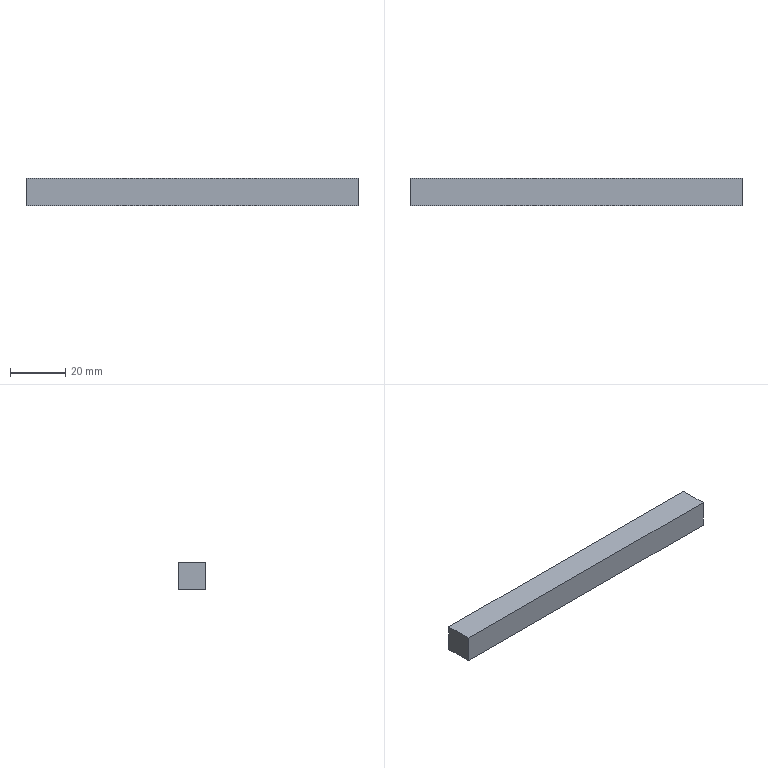Part | STEP file | X-Axis Clamp Block 1 | 1 solid | 6 faces | box 120 x 10 x 10 mm | volume 12000 mm3 | plane 6
STEP:
#1=CARTESIAN_POINT('',(160.919,-17.57,10.));
#2=VERTEX_POINT('',#1);
#3=CARTESIAN_POINT('',(160.919,-17.57,0.));
#4=VERTEX_POINT('',#3);
#5=CARTESIAN_POINT('',(160.919,-17.57,10.));
#6=DIRECTION('',(0.,0.,-1.));
#7=VECTOR('',#6,1000.);
#8=LINE('',#5,#7);
#9=EDGE_CURVE('',#2,#4,#8,.T.);
#10=ORIENTED_EDGE('',*,*,#9,.F.);
#11=CARTESIAN_POINT('',(40.919,-17.57,10.));
#12=VERTEX_POINT('',#11);
#13=CARTESIAN_POINT('',(40.919,-17.57,10.));
#14=DIRECTION('',(1.,0.,0.));
#15=VECTOR('',#14,1000.);
#16=LINE('',#13,#15);
#17=EDGE_CURVE('',#12,#2,#16,.T.);
#18=ORIENTED_EDGE('',*,*,#17,.F.);
#19=CARTESIAN_POINT('',(40.919,-17.57,0.));
#20=VERTEX_POINT('',#19);
#21=CARTESIAN_POINT('',(40.919,-17.57,10.));
#22=DIRECTION('',(0.,0.,1.));
#23=VECTOR('',#22,1000.);
#24=LINE('',#21,#23);
#25=EDGE_CURVE('',#20,#12,#24,.T.);
#26=ORIENTED_EDGE('',*,*,#25,.F.);
#27=CARTESIAN_POINT('',(40.919,-17.57,0.));
#28=DIRECTION('',(-1.,0.,0.));
#29=VECTOR('',#28,1000.);
#30=LINE('',#27,#29);
#31=EDGE_CURVE('',#4,#20,#30,.T.);
#32=ORIENTED_EDGE('',*,*,#31,.F.);
#33=EDGE_LOOP('',(#10,#18,#26,#32));
#34=FACE_OUTER_BOUND('',#33,.T.);
#35=CARTESIAN_POINT('',(40.919,-17.57,10.));
#36=DIRECTION('',(0.,1.,0.));
#37=DIRECTION('',(-1.,0.,0.));
#38=AXIS2_PLACEMENT_3D('',#35,#36,#37);
#39=PLANE('',#38);
#40=ADVANCED_FACE('',(#34),#39,.F.);
#41=CARTESIAN_POINT('',(160.919,-7.57,0.));
#42=VERTEX_POINT('',#41);
#43=CARTESIAN_POINT('',(40.919,-7.57,0.));
#44=VERTEX_POINT('',#43);
#45=CARTESIAN_POINT('',(0.,-7.57,0.));
#46=DIRECTION('',(-1.,0.,0.));
#47=VECTOR('',#46,1000.);
#48=LINE('',#45,#47);
#49=EDGE_CURVE('',#42,#44,#48,.T.);
#50=ORIENTED_EDGE('',*,*,#49,.F.);
#51=CARTESIAN_POINT('',(160.919,0.,0.));
#52=DIRECTION('',(0.,1.,0.));
#53=VECTOR('',#52,1000.);
#54=LINE('',#51,#53);
#55=EDGE_CURVE('',#4,#42,#54,.T.);
#56=ORIENTED_EDGE('',*,*,#55,.F.);
#57=ORIENTED_EDGE('',*,*,#31,.T.);
#58=CARTESIAN_POINT('',(40.919,0.,0.));
#59=DIRECTION('',(0.,-1.,0.));
#60=VECTOR('',#59,1000.);
#61=LINE('',#58,#60);
#62=EDGE_CURVE('',#44,#20,#61,.T.);
#63=ORIENTED_EDGE('',*,*,#62,.F.);
#64=EDGE_LOOP('',(#50,#56,#57,#63));
#65=FACE_OUTER_BOUND('',#64,.T.);
#66=CARTESIAN_POINT('',(0.,0.,0.));
#67=DIRECTION('',(0.,0.,1.));
#68=DIRECTION('',(1.,0.,0.));
#69=AXIS2_PLACEMENT_3D('',#66,#67,#68);
#70=PLANE('',#69);
#71=ADVANCED_FACE('',(#65),#70,.F.);
#72=CARTESIAN_POINT('',(160.919,-7.57,10.));
#73=VERTEX_POINT('',#72);
#74=CARTESIAN_POINT('',(160.919,-7.57,10.));
#75=DIRECTION('',(0.,0.,-1.));
#76=VECTOR('',#75,1000.);
#77=LINE('',#74,#76);
#78=EDGE_CURVE('',#73,#42,#77,.T.);
#79=ORIENTED_EDGE('',*,*,#78,.F.);
#80=CARTESIAN_POINT('',(160.919,-7.57,10.));
#81=DIRECTION('',(0.,1.,0.));
#82=VECTOR('',#81,1000.);
#83=LINE('',#80,#82);
#84=EDGE_CURVE('',#2,#73,#83,.T.);
#85=ORIENTED_EDGE('',*,*,#84,.F.);
#86=ORIENTED_EDGE('',*,*,#9,.T.);
#87=ORIENTED_EDGE('',*,*,#55,.T.);
#88=EDGE_LOOP('',(#79,#85,#86,#87));
#89=FACE_OUTER_BOUND('',#88,.T.);
#90=CARTESIAN_POINT('',(160.919,-7.57,10.));
#91=DIRECTION('',(-1.,0.,0.));
#92=DIRECTION('',(0.,0.,1.));
#93=AXIS2_PLACEMENT_3D('',#90,#91,#92);
#94=PLANE('',#93);
#95=ADVANCED_FACE('',(#89),#94,.F.);
#96=ORIENTED_EDGE('',*,*,#84,.T.);
#97=CARTESIAN_POINT('',(40.919,-7.57,10.));
#98=VERTEX_POINT('',#97);
#99=CARTESIAN_POINT('',(0.,-7.57,10.));
#100=DIRECTION('',(-1.,0.,0.));
#101=VECTOR('',#100,1000.);
#102=LINE('',#99,#101);
#103=EDGE_CURVE('',#73,#98,#102,.T.);
#104=ORIENTED_EDGE('',*,*,#103,.T.);
#105=CARTESIAN_POINT('',(40.919,0.,10.));
#106=DIRECTION('',(0.,-1.,0.));
#107=VECTOR('',#106,1000.);
#108=LINE('',#105,#107);
#109=EDGE_CURVE('',#98,#12,#108,.T.);
#110=ORIENTED_EDGE('',*,*,#109,.T.);
#111=ORIENTED_EDGE('',*,*,#17,.T.);
#112=EDGE_LOOP('',(#96,#104,#110,#111));
#113=FACE_OUTER_BOUND('',#112,.T.);
#114=CARTESIAN_POINT('',(0.,0.,10.));
#115=DIRECTION('',(0.,0.,1.));
#116=DIRECTION('',(1.,0.,0.));
#117=AXIS2_PLACEMENT_3D('',#114,#115,#116);
#118=PLANE('',#117);
#119=ADVANCED_FACE('',(#113),#118,.T.);
#120=ORIENTED_EDGE('',*,*,#25,.T.);
#121=ORIENTED_EDGE('',*,*,#109,.F.);
#122=CARTESIAN_POINT('',(40.919,-7.57,10.));
#123=DIRECTION('',(0.,0.,1.));
#124=VECTOR('',#123,1000.);
#125=LINE('',#122,#124);
#126=EDGE_CURVE('',#44,#98,#125,.T.);
#127=ORIENTED_EDGE('',*,*,#126,.F.);
#128=ORIENTED_EDGE('',*,*,#62,.T.);
#129=EDGE_LOOP('',(#120,#121,#127,#128));
#130=FACE_OUTER_BOUND('',#129,.T.);
#131=CARTESIAN_POINT('',(40.919,-7.57,10.));
#132=DIRECTION('',(1.,0.,0.));
#133=DIRECTION('',(0.,0.,-1.));
#134=AXIS2_PLACEMENT_3D('',#131,#132,#133);
#135=PLANE('',#134);
#136=ADVANCED_FACE('',(#130),#135,.F.);
#137=ORIENTED_EDGE('',*,*,#126,.T.);
#138=ORIENTED_EDGE('',*,*,#103,.F.);
#139=ORIENTED_EDGE('',*,*,#78,.T.);
#140=ORIENTED_EDGE('',*,*,#49,.T.);
#141=EDGE_LOOP('',(#137,#138,#139,#140));
#142=FACE_OUTER_BOUND('',#141,.T.);
#143=CARTESIAN_POINT('',(40.919,-7.57,10.));
#144=DIRECTION('',(0.,-1.,0.));
#145=DIRECTION('',(0.,0.,-1.));
#146=AXIS2_PLACEMENT_3D('',#143,#144,#145);
#147=PLANE('',#146);
#148=ADVANCED_FACE('',(#142),#147,.F.);
#149=CLOSED_SHELL('',(#40,#71,#95,#119,#136,#148));
#150=MANIFOLD_SOLID_BREP('',#149);
#151=CARTESIAN_POINT('',(0.,0.,0.));
#152=DIRECTION('',(0.,0.,1.));
#153=DIRECTION('',(1.,0.,0.));
#154=AXIS2_PLACEMENT_3D('',#151,#152,#153);
#155=(LENGTH_UNIT()NAMED_UNIT(*)SI_UNIT(.MILLI.,.METRE.));
#156=UNCERTAINTY_MEASURE_WITH_UNIT(LENGTH_MEASURE(0.00001),#155,'','');
#157=(NAMED_UNIT(*)PLANE_ANGLE_UNIT()SI_UNIT($,.RADIAN.));
#158=(NAMED_UNIT(*)SI_UNIT($,.STERADIAN.)SOLID_ANGLE_UNIT());
#159=(GEOMETRIC_REPRESENTATION_CONTEXT(3)GLOBAL_UNCERTAINTY_ASSIGNED_CONTEXT((#156))GLOBAL_UNIT_ASSIGNED_CONTEXT((#155,#157,#158))REPRESENTATION_CONTEXT('',''));
#160=ADVANCED_BREP_SHAPE_REPRESENTATION('',(#150,#154),#159);